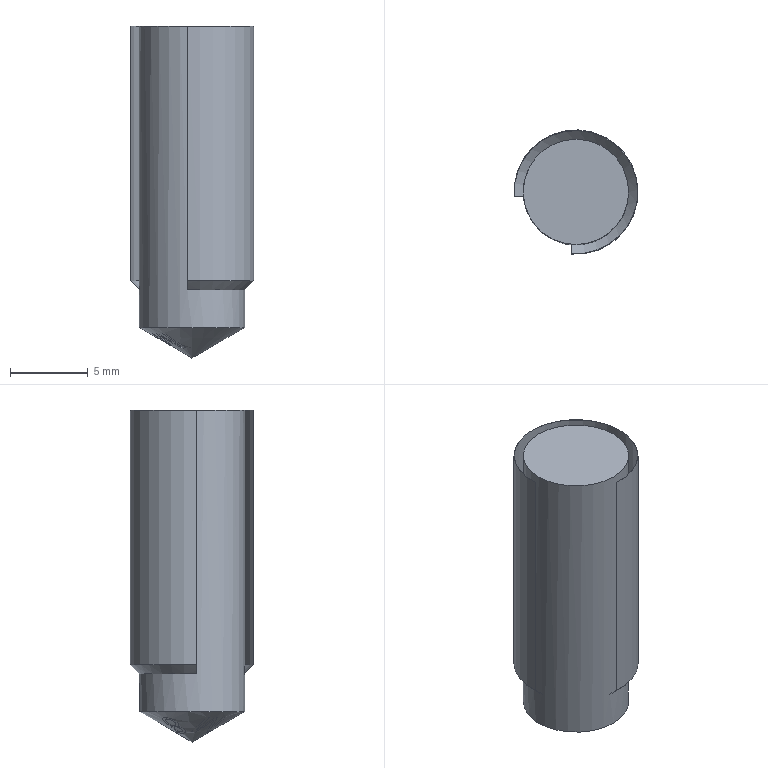Part | STEP file | SOLID | 1 solid | 36 faces | box 8 x 8 x 21.416 mm | volume 734.263 mm3 | plane 17 | other 9 | cone 7 | cylinder 3 | commonest cylinder face diameters 6.8 x1 7.973 x1 8 x1